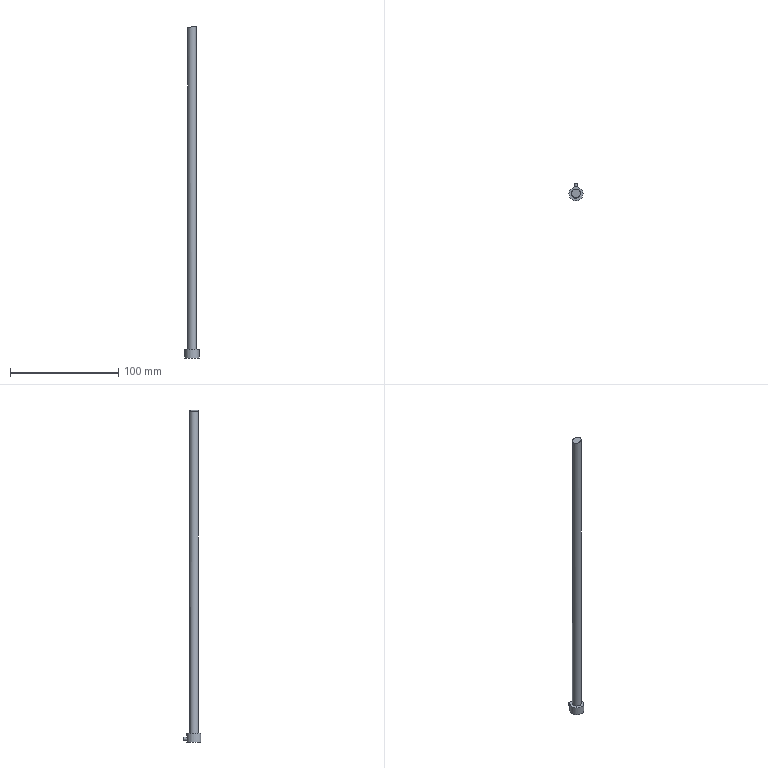Part | STEP file | E108-12-310 | 1 solid | 8 faces | box 13 x 16.5 x 306.86 mm | volume 16065 mm3 | cylinder 3 | plane 3 | spline 1 | cone 1 | commonest cylinder face diameters 3 x1 8 x1 13 x1
STEP:
#1=CARTESIAN_POINT('',(0.,0.,0.));
#2=DIRECTION('',(0.,0.,1.));
#3=DIRECTION('',(1.,0.,0.));
#4=AXIS2_PLACEMENT_3D('',#1,#2,#3);
#5=CARTESIAN_POINT('',(-3.952,0.6196,305.059));
#6=VERTEX_POINT('',#5);
#7=CARTESIAN_POINT('',(-3.952,0.6196,305.059));
#8=CARTESIAN_POINT('',(-4.02,0.1862,305.06));
#9=CARTESIAN_POINT('',(-4.015,-0.2646,305.079));
#10=CARTESIAN_POINT('',(-3.939,-0.6952,305.115));
#11=CARTESIAN_POINT('',(-3.863,-1.126,305.15));
#12=CARTESIAN_POINT('',(-3.714,-1.548,305.203));
#13=CARTESIAN_POINT('',(-3.505,-1.928,305.268));
#14=CARTESIAN_POINT('',(-3.293,-2.313,305.333));
#15=CARTESIAN_POINT('',(-3.015,-2.665,305.413));
#16=CARTESIAN_POINT('',(-2.692,-2.958,305.5));
#17=CARTESIAN_POINT('',(-2.362,-3.259,305.589));
#18=CARTESIAN_POINT('',(-1.976,-3.506,305.688));
#19=CARTESIAN_POINT('',(-1.566,-3.681,305.789));
#20=CARTESIAN_POINT('',(-1.147,-3.859,305.891));
#21=CARTESIAN_POINT('',(-0.6922,-3.966,305.998));
#22=CARTESIAN_POINT('',(-0.2376,-3.993,306.1));
#23=CARTESIAN_POINT('',(0.2209,-4.02,306.203));
#24=CARTESIAN_POINT('',(0.6917,-3.967,306.304));
#25=CARTESIAN_POINT('',(1.135,-3.836,306.395));
#26=CARTESIAN_POINT('',(1.574,-3.706,306.485));
#27=CARTESIAN_POINT('',(1.998,-3.496,306.567));
#28=CARTESIAN_POINT('',(2.37,-3.222,306.635));
#29=CARTESIAN_POINT('',(2.734,-2.954,306.701));
#30=CARTESIAN_POINT('',(3.058,-2.618,306.755));
#31=CARTESIAN_POINT('',(3.313,-2.241,306.793));
#32=CARTESIAN_POINT('',(3.563,-1.872,306.83));
#33=CARTESIAN_POINT('',(3.753,-1.454,306.852));
#34=CARTESIAN_POINT('',(3.867,-1.023,306.858));
#35=CARTESIAN_POINT('',(3.979,-0.5976,306.864));
#36=CARTESIAN_POINT('',(4.021,-0.1473,306.855));
#37=CARTESIAN_POINT('',(3.989,0.2907,306.83));
#38=CARTESIAN_POINT('',(3.958,0.7275,306.806));
#39=CARTESIAN_POINT('',(3.852,1.164,306.767));
#40=CARTESIAN_POINT('',(3.681,1.565,306.716));
#41=CARTESIAN_POINT('',(3.509,1.97,306.664));
#42=CARTESIAN_POINT('',(3.267,2.35,306.599));
#43=CARTESIAN_POINT('',(2.974,2.674,306.525));
#44=CARTESIAN_POINT('',(2.677,3.005,306.449));
#45=CARTESIAN_POINT('',(2.32,3.288,306.363));
#46=CARTESIAN_POINT('',(1.933,3.502,306.272));
#47=CARTESIAN_POINT('',(1.538,3.72,306.179));
#48=CARTESIAN_POINT('',(1.101,3.872,306.078));
#49=CARTESIAN_POINT('',(0.657,3.946,305.978));
#50=CARTESIAN_POINT('',(0.2063,4.021,305.876));
#51=CARTESIAN_POINT('',(-0.2635,4.017,305.772));
#52=CARTESIAN_POINT('',(-0.7138,3.936,305.674));
#53=CARTESIAN_POINT('',(-1.165,3.854,305.576));
#54=CARTESIAN_POINT('',(-1.61,3.691,305.481));
#55=CARTESIAN_POINT('',(-2.01,3.459,305.399));
#56=CARTESIAN_POINT('',(-2.404,3.229,305.317));
#57=CARTESIAN_POINT('',(-2.765,2.926,305.245));
#58=CARTESIAN_POINT('',(-3.062,2.574,305.19));
#59=CARTESIAN_POINT('',(-3.35,2.231,305.136));
#60=CARTESIAN_POINT('',(-3.585,1.831,305.097));
#61=CARTESIAN_POINT('',(-3.744,1.408,305.076));
#62=CARTESIAN_POINT('',(-3.84,1.154,305.064));
#63=CARTESIAN_POINT('',(-3.91,0.8882,305.058));
#64=CARTESIAN_POINT('',(-3.952,0.6196,305.059));
#65=B_SPLINE_CURVE_WITH_KNOTS('',3,(#7,#8,#9,#10,#11,#12,#13,#14,#15,#16,#17,#18,#19,#20,#21,#22,#23,#24,#25,#26,#27,#28,#29,#30,#31,#32,#33,#34,#35,#36,#37,#38,#39,#40,#41,#42,#43,#44,#45,#46,#47,#48,#49,#50,#51,#52,#53,#54,#55,#56,#57,#58,#59,#60,#61,#62,#63,#64),.UNSPECIFIED.,.T.,.F.,(1,3,3,3,3,3,3,3,3,3,3,3,3,3,3,3,3,3,3,3,3,1),(-0.03191,0.,0.05196,0.1039,0.1565,0.2105,0.2658,0.3216,0.3769,0.4311,0.484,0.5361,0.588,0.6405,0.6939,0.7485,0.804,0.8596,0.9145,0.9681,1.,1.052),.UNSPECIFIED.);
#66=CARTESIAN_POINT('',(0.,0.,108.));
#67=DIRECTION('',(0.,0.,-1.));
#68=DIRECTION('',(-1.,0.,0.));
#69=AXIS2_PLACEMENT_3D('',#66,#67,#68);
#70=CYLINDRICAL_SURFACE('',#69,4.);
#71=CARTESIAN_POINT('',(6.439,-197.059));
#72=CARTESIAN_POINT('',(6.415,-197.059));
#73=CARTESIAN_POINT('',(6.367,-197.061));
#74=CARTESIAN_POINT('',(6.294,-197.07));
#75=CARTESIAN_POINT('',(6.222,-197.083));
#76=CARTESIAN_POINT('',(6.15,-197.101));
#77=CARTESIAN_POINT('',(6.078,-197.124));
#78=CARTESIAN_POINT('',(6.006,-197.152));
#79=CARTESIAN_POINT('',(5.934,-197.185));
#80=CARTESIAN_POINT('',(5.862,-197.221));
#81=CARTESIAN_POINT('',(5.79,-197.261));
#82=CARTESIAN_POINT('',(5.719,-197.305));
#83=CARTESIAN_POINT('',(5.648,-197.353));
#84=CARTESIAN_POINT('',(5.576,-197.403));
#85=CARTESIAN_POINT('',(5.505,-197.457));
#86=CARTESIAN_POINT('',(5.435,-197.513));
#87=CARTESIAN_POINT('',(5.364,-197.571));
#88=CARTESIAN_POINT('',(5.293,-197.631));
#89=CARTESIAN_POINT('',(5.222,-197.693));
#90=CARTESIAN_POINT('',(5.152,-197.755));
#91=CARTESIAN_POINT('',(5.081,-197.819));
#92=CARTESIAN_POINT('',(5.011,-197.883));
#93=CARTESIAN_POINT('',(4.94,-197.947));
#94=CARTESIAN_POINT('',(4.87,-198.012));
#95=CARTESIAN_POINT('',(4.799,-198.076));
#96=CARTESIAN_POINT('',(4.729,-198.139));
#97=CARTESIAN_POINT('',(4.658,-198.201));
#98=CARTESIAN_POINT('',(4.588,-198.262));
#99=CARTESIAN_POINT('',(4.517,-198.321));
#100=CARTESIAN_POINT('',(4.446,-198.379));
#101=CARTESIAN_POINT('',(4.375,-198.434));
#102=CARTESIAN_POINT('',(4.304,-198.486));
#103=CARTESIAN_POINT('',(4.233,-198.537));
#104=CARTESIAN_POINT('',(4.162,-198.584));
#105=CARTESIAN_POINT('',(4.09,-198.628));
#106=CARTESIAN_POINT('',(4.019,-198.669));
#107=CARTESIAN_POINT('',(3.947,-198.706));
#108=CARTESIAN_POINT('',(3.875,-198.74));
#109=CARTESIAN_POINT('',(3.803,-198.769));
#110=CARTESIAN_POINT('',(3.732,-198.795));
#111=CARTESIAN_POINT('',(3.66,-198.816));
#112=CARTESIAN_POINT('',(3.587,-198.834));
#113=CARTESIAN_POINT('',(3.515,-198.847));
#114=CARTESIAN_POINT('',(3.443,-198.856));
#115=CARTESIAN_POINT('',(3.371,-198.86));
#116=CARTESIAN_POINT('',(3.298,-198.86));
#117=CARTESIAN_POINT('',(3.226,-198.856));
#118=CARTESIAN_POINT('',(3.153,-198.847));
#119=CARTESIAN_POINT('',(3.081,-198.834));
#120=CARTESIAN_POINT('',(3.009,-198.817));
#121=CARTESIAN_POINT('',(2.937,-198.795));
#122=CARTESIAN_POINT('',(2.865,-198.77));
#123=CARTESIAN_POINT('',(2.793,-198.741));
#124=CARTESIAN_POINT('',(2.721,-198.708));
#125=CARTESIAN_POINT('',(2.65,-198.672));
#126=CARTESIAN_POINT('',(2.578,-198.632));
#127=CARTESIAN_POINT('',(2.506,-198.589));
#128=CARTESIAN_POINT('',(2.435,-198.543));
#129=CARTESIAN_POINT('',(2.364,-198.494));
#130=CARTESIAN_POINT('',(2.293,-198.443));
#131=CARTESIAN_POINT('',(2.221,-198.389));
#132=CARTESIAN_POINT('',(2.15,-198.333));
#133=CARTESIAN_POINT('',(2.08,-198.276));
#134=CARTESIAN_POINT('',(2.009,-198.217));
#135=CARTESIAN_POINT('',(1.938,-198.156));
#136=CARTESIAN_POINT('',(1.868,-198.095));
#137=CARTESIAN_POINT('',(1.797,-198.032));
#138=CARTESIAN_POINT('',(1.727,-197.97));
#139=CARTESIAN_POINT('',(1.656,-197.907));
#140=CARTESIAN_POINT('',(1.585,-197.844));
#141=CARTESIAN_POINT('',(1.515,-197.781));
#142=CARTESIAN_POINT('',(1.444,-197.719));
#143=CARTESIAN_POINT('',(1.374,-197.659));
#144=CARTESIAN_POINT('',(1.303,-197.599));
#145=CARTESIAN_POINT('',(1.232,-197.541));
#146=CARTESIAN_POINT('',(1.161,-197.485));
#147=CARTESIAN_POINT('',(1.09,-197.431));
#148=CARTESIAN_POINT('',(1.019,-197.38));
#149=CARTESIAN_POINT('',(0.9481,-197.332));
#150=CARTESIAN_POINT('',(0.8765,-197.286));
#151=CARTESIAN_POINT('',(0.8049,-197.244));
#152=CARTESIAN_POINT('',(0.7332,-197.206));
#153=CARTESIAN_POINT('',(0.6619,-197.172));
#154=CARTESIAN_POINT('',(0.59,-197.142));
#155=CARTESIAN_POINT('',(0.5178,-197.116));
#156=CARTESIAN_POINT('',(0.4455,-197.094));
#157=CARTESIAN_POINT('',(0.3736,-197.078));
#158=CARTESIAN_POINT('',(0.3011,-197.066));
#159=CARTESIAN_POINT('',(0.2282,-197.059));
#160=CARTESIAN_POINT('',(0.1797,-197.058));
#161=CARTESIAN_POINT('',(0.1555,-197.059));
#162=B_SPLINE_CURVE_WITH_KNOTS('',3,(#71,#72,#73,#74,#75,#76,#77,#78,#79,#80,#81,#82,#83,#84,#85,#86,#87,#88,#89,#90,#91,#92,#93,#94,#95,#96,#97,#98,#99,#100,#101,#102,#103,#104,#105,#106,#107,#108,#109,#110,#111,#112,#113,#114,#115,#116,#117,#118,#119,#120,#121,#122,#123,#124,#125,#126,#127,#128,#129,#130,#131,#132,#133,#134,#135,#136,#137,#138,#139,#140,#141,#142,#143,#144,#145,#146,#147,#148,#149,#150,#151,#152,#153,#154,#155,#156,#157,#158,#159,#160,#161),.UNSPECIFIED.,.F.,.F.,(4,1,1,1,1,1,1,1,1,1,1,1,1,1,1,1,1,1,1,1,1,1,1,1,1,1,1,1,1,1,1,1,1,1,1,1,1,1,1,1,1,1,1,1,1,1,1,1,1,1,1,1,1,1,1,1,1,1,1,1,1,1,1,1,1,1,1,1,1,1,1,1,1,1,1,1,1,1,1,1,1,1,1,1,1,1,1,1,4),(0.,0.01136,0.02273,0.03409,0.04545,0.05682,0.06818,0.07955,0.09091,0.1023,0.1136,0.125,0.1364,0.1477,0.1591,0.1705,0.1818,0.1932,0.2045,0.2159,0.2273,0.2386,0.25,0.2614,0.2727,0.2841,0.2955,0.3068,0.3182,0.3295,0.3409,0.3523,0.3636,0.375,0.3864,0.3977,0.4091,0.4205,0.4318,0.4432,0.4545,0.4659,0.4773,0.4886,0.5,0.5114,0.5227,0.5341,0.5455,0.5568,0.5682,0.5795,0.5909,0.6023,0.6136,0.625,0.6364,0.6477,0.6591,0.6705,0.6818,0.6932,0.7045,0.7159,0.7273,0.7386,0.75,0.7614,0.7727,0.7841,0.7955,0.8068,0.8182,0.8295,0.8409,0.8523,0.8636,0.875,0.8864,0.8977,0.9091,0.9205,0.9318,0.9432,0.9545,0.9659,0.9773,0.9886,1.),.QUASI_UNIFORM_KNOTS.);
#163=(GEOMETRIC_REPRESENTATION_CONTEXT(2)PARAMETRIC_REPRESENTATION_CONTEXT()REPRESENTATION_CONTEXT('',''));
#164=DEFINITIONAL_REPRESENTATION('',(#162),#163);
#165=PCURVE('',#70,#164);
#166=CARTESIAN_POINT('',(-7.07,-15.345,304.943));
#167=CARTESIAN_POINT('',(0.4092,-15.342,306.816));
#168=CARTESIAN_POINT('',(7.936,-15.339,308.349));
#169=CARTESIAN_POINT('',(15.537,-15.336,309.52));
#170=CARTESIAN_POINT('',(-7.049,-4.486,304.509));
#171=CARTESIAN_POINT('',(0.4231,-4.483,306.385));
#172=CARTESIAN_POINT('',(7.941,-4.48,307.92));
#173=CARTESIAN_POINT('',(15.534,-4.477,309.095));
#174=CARTESIAN_POINT('',(-7.039,6.373,304.069));
#175=CARTESIAN_POINT('',(0.4255,6.376,305.948));
#176=CARTESIAN_POINT('',(7.935,6.378,307.486));
#177=CARTESIAN_POINT('',(15.519,6.381,308.665));
#178=CARTESIAN_POINT('',(-7.039,17.231,303.624));
#179=CARTESIAN_POINT('',(0.4166,17.233,305.505));
#180=CARTESIAN_POINT('',(7.918,17.236,307.047));
#181=CARTESIAN_POINT('',(15.493,17.239,308.229));
#182=B_SPLINE_SURFACE_WITH_KNOTS('',3,3,((#166,#167,#168,#169),(#170,#171,#172,#173),(#174,#175,#176,#177),(#178,#179,#180,#181)),.UNSPECIFIED.,.F.,.F.,.F.,(4,4),(4,4),(0.,1.),(0.,1.),.PIECEWISE_BEZIER_KNOTS.);
#183=CARTESIAN_POINT('',(0.49,0.138));
#184=CARTESIAN_POINT('',(0.4871,0.1374));
#185=CARTESIAN_POINT('',(0.4812,0.1364));
#186=CARTESIAN_POINT('',(0.4724,0.1358));
#187=CARTESIAN_POINT('',(0.4635,0.1361));
#188=CARTESIAN_POINT('',(0.4546,0.1373));
#189=CARTESIAN_POINT('',(0.4459,0.1395));
#190=CARTESIAN_POINT('',(0.4374,0.1426));
#191=CARTESIAN_POINT('',(0.4289,0.1466));
#192=CARTESIAN_POINT('',(0.4208,0.1514));
#193=CARTESIAN_POINT('',(0.4129,0.157));
#194=CARTESIAN_POINT('',(0.4053,0.1634));
#195=CARTESIAN_POINT('',(0.3981,0.1706));
#196=CARTESIAN_POINT('',(0.3912,0.1785));
#197=CARTESIAN_POINT('',(0.3847,0.1871));
#198=CARTESIAN_POINT('',(0.3788,0.1963));
#199=CARTESIAN_POINT('',(0.3733,0.206));
#200=CARTESIAN_POINT('',(0.3682,0.2163));
#201=CARTESIAN_POINT('',(0.3637,0.2271));
#202=CARTESIAN_POINT('',(0.3597,0.2383));
#203=CARTESIAN_POINT('',(0.3564,0.2498));
#204=CARTESIAN_POINT('',(0.3535,0.2616));
#205=CARTESIAN_POINT('',(0.3513,0.2738));
#206=CARTESIAN_POINT('',(0.3496,0.2861));
#207=CARTESIAN_POINT('',(0.3485,0.2985));
#208=CARTESIAN_POINT('',(0.3481,0.311));
#209=CARTESIAN_POINT('',(0.3483,0.3236));
#210=CARTESIAN_POINT('',(0.349,0.3361));
#211=CARTESIAN_POINT('',(0.3504,0.3485));
#212=CARTESIAN_POINT('',(0.3524,0.3608));
#213=CARTESIAN_POINT('',(0.355,0.3727));
#214=CARTESIAN_POINT('',(0.3581,0.3845));
#215=CARTESIAN_POINT('',(0.3619,0.3959));
#216=CARTESIAN_POINT('',(0.3662,0.407));
#217=CARTESIAN_POINT('',(0.3711,0.4175));
#218=CARTESIAN_POINT('',(0.3764,0.4275));
#219=CARTESIAN_POINT('',(0.3823,0.437));
#220=CARTESIAN_POINT('',(0.3886,0.4459));
#221=CARTESIAN_POINT('',(0.3954,0.4541));
#222=CARTESIAN_POINT('',(0.4025,0.4616));
#223=CARTESIAN_POINT('',(0.4101,0.4683));
#224=CARTESIAN_POINT('',(0.4179,0.4742));
#225=CARTESIAN_POINT('',(0.4261,0.4793));
#226=CARTESIAN_POINT('',(0.4345,0.4836));
#227=CARTESIAN_POINT('',(0.443,0.4869));
#228=CARTESIAN_POINT('',(0.4517,0.4894));
#229=CARTESIAN_POINT('',(0.4606,0.4909));
#230=CARTESIAN_POINT('',(0.4695,0.4915));
#231=CARTESIAN_POINT('',(0.4783,0.4913));
#232=CARTESIAN_POINT('',(0.4871,0.49));
#233=CARTESIAN_POINT('',(0.4959,0.4879));
#234=CARTESIAN_POINT('',(0.5045,0.4848));
#235=CARTESIAN_POINT('',(0.5129,0.4809));
#236=CARTESIAN_POINT('',(0.5211,0.4761));
#237=CARTESIAN_POINT('',(0.529,0.4705));
#238=CARTESIAN_POINT('',(0.5366,0.4641));
#239=CARTESIAN_POINT('',(0.5439,0.4569));
#240=CARTESIAN_POINT('',(0.5507,0.4491));
#241=CARTESIAN_POINT('',(0.5572,0.4406));
#242=CARTESIAN_POINT('',(0.5632,0.4314));
#243=CARTESIAN_POINT('',(0.5687,0.4216));
#244=CARTESIAN_POINT('',(0.5738,0.4113));
#245=CARTESIAN_POINT('',(0.5783,0.4005));
#246=CARTESIAN_POINT('',(0.5822,0.3894));
#247=CARTESIAN_POINT('',(0.5856,0.3778));
#248=CARTESIAN_POINT('',(0.5885,0.3659));
#249=CARTESIAN_POINT('',(0.5907,0.3537));
#250=CARTESIAN_POINT('',(0.5924,0.3415));
#251=CARTESIAN_POINT('',(0.5934,0.329));
#252=CARTESIAN_POINT('',(0.5938,0.3165));
#253=CARTESIAN_POINT('',(0.5937,0.3039));
#254=CARTESIAN_POINT('',(0.5929,0.2913));
#255=CARTESIAN_POINT('',(0.5915,0.279));
#256=CARTESIAN_POINT('',(0.5895,0.2668));
#257=CARTESIAN_POINT('',(0.5869,0.2547));
#258=CARTESIAN_POINT('',(0.5837,0.2429));
#259=CARTESIAN_POINT('',(0.5799,0.2315));
#260=CARTESIAN_POINT('',(0.5757,0.2205));
#261=CARTESIAN_POINT('',(0.5708,0.21));
#262=CARTESIAN_POINT('',(0.5654,0.1999));
#263=CARTESIAN_POINT('',(0.5596,0.1904));
#264=CARTESIAN_POINT('',(0.5532,0.1815));
#265=CARTESIAN_POINT('',(0.5465,0.1733));
#266=CARTESIAN_POINT('',(0.5394,0.1658));
#267=CARTESIAN_POINT('',(0.5318,0.1591));
#268=CARTESIAN_POINT('',(0.524,0.1531));
#269=CARTESIAN_POINT('',(0.5159,0.148));
#270=CARTESIAN_POINT('',(0.5074,0.1437));
#271=CARTESIAN_POINT('',(0.4988,0.1403));
#272=CARTESIAN_POINT('',(0.493,0.1387));
#273=CARTESIAN_POINT('',(0.49,0.138));
#274=B_SPLINE_CURVE_WITH_KNOTS('',3,(#183,#184,#185,#186,#187,#188,#189,#190,#191,#192,#193,#194,#195,#196,#197,#198,#199,#200,#201,#202,#203,#204,#205,#206,#207,#208,#209,#210,#211,#212,#213,#214,#215,#216,#217,#218,#219,#220,#221,#222,#223,#224,#225,#226,#227,#228,#229,#230,#231,#232,#233,#234,#235,#236,#237,#238,#239,#240,#241,#242,#243,#244,#245,#246,#247,#248,#249,#250,#251,#252,#253,#254,#255,#256,#257,#258,#259,#260,#261,#262,#263,#264,#265,#266,#267,#268,#269,#270,#271,#272,#273),.UNSPECIFIED.,.T.,.F.,(4,1,1,1,1,1,1,1,1,1,1,1,1,1,1,1,1,1,1,1,1,1,1,1,1,1,1,1,1,1,1,1,1,1,1,1,1,1,1,1,1,1,1,1,1,1,1,1,1,1,1,1,1,1,1,1,1,1,1,1,1,1,1,1,1,1,1,1,1,1,1,1,1,1,1,1,1,1,1,1,1,1,1,1,1,1,1,1,4),(0.,0.01136,0.02273,0.03409,0.04545,0.05682,0.06818,0.07955,0.09091,0.1023,0.1136,0.125,0.1364,0.1477,0.1591,0.1705,0.1818,0.1932,0.2045,0.2159,0.2273,0.2386,0.25,0.2614,0.2727,0.2841,0.2955,0.3068,0.3182,0.3295,0.3409,0.3523,0.3636,0.375,0.3864,0.3977,0.4091,0.4205,0.4318,0.4432,0.4545,0.4659,0.4773,0.4886,0.5,0.5114,0.5227,0.5341,0.5455,0.5568,0.5682,0.5795,0.5909,0.6023,0.6136,0.625,0.6364,0.6477,0.6591,0.6705,0.6818,0.6932,0.7045,0.7159,0.7273,0.7386,0.75,0.7614,0.7727,0.7841,0.7955,0.8068,0.8182,0.8295,0.8409,0.8523,0.8636,0.875,0.8864,0.8977,0.9091,0.9205,0.9318,0.9432,0.9545,0.9659,0.9773,0.9886,1.),.QUASI_UNIFORM_KNOTS.);
#275=(GEOMETRIC_REPRESENTATION_CONTEXT(2)PARAMETRIC_REPRESENTATION_CONTEXT()REPRESENTATION_CONTEXT('',''));
#276=DEFINITIONAL_REPRESENTATION('',(#274),#275);
#277=PCURVE('',#182,#276);
#278=SURFACE_CURVE('',#65,(#165,#277),.PCURVE_S1.);
#279=EDGE_CURVE('',#6,#6,#278,.T.);
#280=ORIENTED_EDGE('',*,*,#279,.F.);
#281=CARTESIAN_POINT('',(-3.952,0.6196,8.));
#282=VERTEX_POINT('',#281);
#283=CARTESIAN_POINT('',(-3.952,0.6196,305.059));
#284=CARTESIAN_POINT('',(-3.952,0.6196,8.));
#285=B_SPLINE_CURVE_WITH_KNOTS('',1,(#283,#284),.UNSPECIFIED.,.F.,.F.,(2,2),(-197.059,100.),.PIECEWISE_BEZIER_KNOTS.);
#286=CARTESIAN_POINT('',(6.439,0.));
#287=DIRECTION('',(0.,1.));
#288=VECTOR('',#287,1.);
#289=LINE('',#286,#288);
#290=(GEOMETRIC_REPRESENTATION_CONTEXT(2)PARAMETRIC_REPRESENTATION_CONTEXT()REPRESENTATION_CONTEXT('',''));
#291=DEFINITIONAL_REPRESENTATION('',(#289),#290);
#292=PCURVE('',#70,#291);
#293=CARTESIAN_POINT('',(0.1555,0.));
#294=DIRECTION('',(0.,1.));
#295=VECTOR('',#294,1.);
#296=LINE('',#293,#295);
#297=(GEOMETRIC_REPRESENTATION_CONTEXT(2)PARAMETRIC_REPRESENTATION_CONTEXT()REPRESENTATION_CONTEXT('',''));
#298=DEFINITIONAL_REPRESENTATION('',(#296),#297);
#299=PCURVE('',#70,#298);
#300=SEAM_CURVE('',#285,(#292,#299),.PCURVE_S1.);
#301=EDGE_CURVE('',#6,#282,#300,.T.);
#302=ORIENTED_EDGE('',*,*,#301,.T.);
#303=CARTESIAN_POINT('',(4.,0.,8.));
#304=VERTEX_POINT('',#303);
#305=CARTESIAN_POINT('',(0.,0.,8.));
#306=DIRECTION('',(0.,0.,1.));
#307=DIRECTION('',(1.,0.,0.));
#308=AXIS2_PLACEMENT_3D('',#305,#306,#307);
#309=CIRCLE('',#308,4.);
#310=CARTESIAN_POINT('',(9.425,100.));
#311=DIRECTION('',(-1.,0.));
#312=VECTOR('',#311,1.);
#313=LINE('',#310,#312);
#314=(GEOMETRIC_REPRESENTATION_CONTEXT(2)PARAMETRIC_REPRESENTATION_CONTEXT()REPRESENTATION_CONTEXT('',''));
#315=DEFINITIONAL_REPRESENTATION('',(#313),#314);
#316=PCURVE('',#70,#315);
#317=CARTESIAN_POINT('',(0.,0.,8.));
#318=DIRECTION('',(0.,0.,-1.));
#319=DIRECTION('',(1.,0.,0.));
#320=AXIS2_PLACEMENT_3D('',#317,#318,#319);
#321=PLANE('',#320);
#322=CARTESIAN_POINT('',(4.,0.));
#323=CARTESIAN_POINT('',(4.,-6.928));
#324=CARTESIAN_POINT('',(-2.,-3.464));
#325=CARTESIAN_POINT('',(-8.,0.));
#326=CARTESIAN_POINT('',(-2.,3.464));
#327=CARTESIAN_POINT('',(4.,6.928));
#328=CARTESIAN_POINT('',(4.,0.));
#329=(BOUNDED_CURVE()B_SPLINE_CURVE(2,(#322,#323,#324,#325,#326,#327,#328),.UNSPECIFIED.,.T.,.F.)B_SPLINE_CURVE_WITH_KNOTS((1,2,2,2,2,1),(-2.094,0.,2.094,4.189,6.283,8.378),.UNSPECIFIED.)CURVE()GEOMETRIC_REPRESENTATION_ITEM()RATIONAL_B_SPLINE_CURVE((1.,0.5,1.,0.5,1.,0.5,1.))REPRESENTATION_ITEM(''));
#330=(GEOMETRIC_REPRESENTATION_CONTEXT(2)PARAMETRIC_REPRESENTATION_CONTEXT()REPRESENTATION_CONTEXT('',''));
#331=DEFINITIONAL_REPRESENTATION('',(#329),#330);
#332=PCURVE('',#321,#331);
#333=SURFACE_CURVE('',#309,(#316,#332),.PCURVE_S1.);
#334=EDGE_CURVE('',#282,#304,#333,.T.);
#335=ORIENTED_EDGE('',*,*,#334,.T.);
#336=CARTESIAN_POINT('',(0.,0.,8.));
#337=DIRECTION('',(0.,0.,1.));
#338=DIRECTION('',(1.,0.,0.));
#339=AXIS2_PLACEMENT_3D('',#336,#337,#338);
#340=CIRCLE('',#339,4.);
#341=CARTESIAN_POINT('',(3.142,100.));
#342=DIRECTION('',(-1.,0.));
#343=VECTOR('',#342,1.);
#344=LINE('',#341,#343);
#345=(GEOMETRIC_REPRESENTATION_CONTEXT(2)PARAMETRIC_REPRESENTATION_CONTEXT()REPRESENTATION_CONTEXT('',''));
#346=DEFINITIONAL_REPRESENTATION('',(#344),#345);
#347=PCURVE('',#70,#346);
#348=CARTESIAN_POINT('',(4.,0.));
#349=CARTESIAN_POINT('',(4.,-6.928));
#350=CARTESIAN_POINT('',(-2.,-3.464));
#351=CARTESIAN_POINT('',(-8.,0.));
#352=CARTESIAN_POINT('',(-2.,3.464));
#353=CARTESIAN_POINT('',(4.,6.928));
#354=CARTESIAN_POINT('',(4.,0.));
#355=(BOUNDED_CURVE()B_SPLINE_CURVE(2,(#348,#349,#350,#351,#352,#353,#354),.UNSPECIFIED.,.T.,.F.)B_SPLINE_CURVE_WITH_KNOTS((1,2,2,2,2,1),(-2.094,0.,2.094,4.189,6.283,8.378),.UNSPECIFIED.)CURVE()GEOMETRIC_REPRESENTATION_ITEM()RATIONAL_B_SPLINE_CURVE((1.,0.5,1.,0.5,1.,0.5,1.))REPRESENTATION_ITEM(''));
#356=(GEOMETRIC_REPRESENTATION_CONTEXT(2)PARAMETRIC_REPRESENTATION_CONTEXT()REPRESENTATION_CONTEXT('',''));
#357=DEFINITIONAL_REPRESENTATION('',(#355),#356);
#358=PCURVE('',#321,#357);
#359=SURFACE_CURVE('',#340,(#347,#358),.PCURVE_S1.);
#360=EDGE_CURVE('',#304,#282,#359,.T.);
#361=ORIENTED_EDGE('',*,*,#360,.T.);
#362=ORIENTED_EDGE('',*,*,#301,.F.);
#363=EDGE_LOOP('',(#280,#302,#335,#361,#362));
#364=FACE_BOUND('',#363,.T.);
#365=ADVANCED_FACE('',(#364),#70,.T.);
#366=ORIENTED_EDGE('',*,*,#279,.F.);
#367=EDGE_LOOP('',(#366));
#368=FACE_BOUND('',#367,.F.);
#369=ADVANCED_FACE('',(#368),#182,.F.);
#370=CARTESIAN_POINT('',(6.5,0.,0.));
#371=VERTEX_POINT('',#370);
#372=CARTESIAN_POINT('',(-6.5,0.,0.));
#373=VERTEX_POINT('',#372);
#374=CARTESIAN_POINT('',(0.,0.,0.));
#375=DIRECTION('',(0.,0.,-1.));
#376=DIRECTION('',(-1.,0.,0.));
#377=AXIS2_PLACEMENT_3D('',#374,#375,#376);
#378=CIRCLE('',#377,6.5);
#379=CARTESIAN_POINT('',(0.,0.,8.));
#380=DIRECTION('',(0.,0.,-1.));
#381=DIRECTION('',(1.,0.,0.));
#382=AXIS2_PLACEMENT_3D('',#379,#380,#381);
#383=CYLINDRICAL_SURFACE('',#382,6.5);
#384=CARTESIAN_POINT('',(-3.142,8.));
#385=DIRECTION('',(1.,0.));
#386=VECTOR('',#385,1.);
#387=LINE('',#384,#386);
#388=(GEOMETRIC_REPRESENTATION_CONTEXT(2)PARAMETRIC_REPRESENTATION_CONTEXT()REPRESENTATION_CONTEXT('',''));
#389=DEFINITIONAL_REPRESENTATION('',(#387),#388);
#390=PCURVE('',#383,#389);
#391=CARTESIAN_POINT('',(240.,-1000.,0.));
#392=DIRECTION('',(0.,0.,1.));
#393=DIRECTION('',(-1.,0.,0.));
#394=AXIS2_PLACEMENT_3D('',#391,#392,#393);
#395=PLANE('',#394);
#396=CARTESIAN_POINT('',(246.5,-1000.));
#397=CARTESIAN_POINT('',(246.5,-1011.258));
#398=CARTESIAN_POINT('',(236.75,-1005.629));
#399=CARTESIAN_POINT('',(227.,-1000.));
#400=CARTESIAN_POINT('',(236.75,-994.371));
#401=CARTESIAN_POINT('',(246.5,-988.742));
#402=CARTESIAN_POINT('',(246.5,-1000.));
#403=(BOUNDED_CURVE()B_SPLINE_CURVE(2,(#396,#397,#398,#399,#400,#401,#402),.UNSPECIFIED.,.T.,.F.)B_SPLINE_CURVE_WITH_KNOTS((1,2,2,2,2,1),(-2.094,0.,2.094,4.189,6.283,8.378),.UNSPECIFIED.)CURVE()GEOMETRIC_REPRESENTATION_ITEM()RATIONAL_B_SPLINE_CURVE((1.,0.5,1.,0.5,1.,0.5,1.))REPRESENTATION_ITEM(''));
#404=(GEOMETRIC_REPRESENTATION_CONTEXT(2)PARAMETRIC_REPRESENTATION_CONTEXT()REPRESENTATION_CONTEXT('',''));
#405=DEFINITIONAL_REPRESENTATION('',(#403),#404);
#406=PCURVE('',#395,#405);
#407=SURFACE_CURVE('',#378,(#390,#406),.PCURVE_S1.);
#408=EDGE_CURVE('',#371,#373,#407,.T.);
#409=ORIENTED_EDGE('',*,*,#408,.F.);
#410=CARTESIAN_POINT('',(6.5,0.,8.));
#411=VERTEX_POINT('',#410);
#412=CARTESIAN_POINT('',(6.5,0.,8.));
#413=CARTESIAN_POINT('',(6.5,0.,0.));
#414=B_SPLINE_CURVE_WITH_KNOTS('',1,(#412,#413),.UNSPECIFIED.,.F.,.F.,(2,2),(0.,8.),.PIECEWISE_BEZIER_KNOTS.);
#415=CARTESIAN_POINT('',(0.,0.));
#416=DIRECTION('',(0.,1.));
#417=VECTOR('',#416,1.);
#418=LINE('',#415,#417);
#419=(GEOMETRIC_REPRESENTATION_CONTEXT(2)PARAMETRIC_REPRESENTATION_CONTEXT()REPRESENTATION_CONTEXT('',''));
#420=DEFINITIONAL_REPRESENTATION('',(#418),#419);
#421=PCURVE('',#383,#420);
#422=CARTESIAN_POINT('',(6.283,0.));
#423=DIRECTION('',(0.,1.));
#424=VECTOR('',#423,1.);
#425=LINE('',#422,#424);
#426=(GEOMETRIC_REPRESENTATION_CONTEXT(2)PARAMETRIC_REPRESENTATION_CONTEXT()REPRESENTATION_CONTEXT('',''));
#427=DEFINITIONAL_REPRESENTATION('',(#425),#426);
#428=PCURVE('',#383,#427);
#429=SEAM_CURVE('',#414,(#421,#428),.PCURVE_S1.);
#430=EDGE_CURVE('',#411,#371,#429,.T.);
#431=ORIENTED_EDGE('',*,*,#430,.F.);
#432=CARTESIAN_POINT('',(0.,0.,8.));
#433=DIRECTION('',(0.,0.,-1.));
#434=DIRECTION('',(1.,0.,0.));
#435=AXIS2_PLACEMENT_3D('',#432,#433,#434);
#436=CIRCLE('',#435,6.5);
#437=CARTESIAN_POINT('',(0.,0.));
#438=DIRECTION('',(1.,0.));
#439=VECTOR('',#438,1.);
#440=LINE('',#437,#439);
#441=(GEOMETRIC_REPRESENTATION_CONTEXT(2)PARAMETRIC_REPRESENTATION_CONTEXT()REPRESENTATION_CONTEXT('',''));
#442=DEFINITIONAL_REPRESENTATION('',(#440),#441);
#443=PCURVE('',#383,#442);
#444=CARTESIAN_POINT('',(0.,0.));
#445=DIRECTION('',(1.,0.));
#446=AXIS2_PLACEMENT_2D('',#444,#445);
#447=CIRCLE('',#446,6.5);
#448=(GEOMETRIC_REPRESENTATION_CONTEXT(2)PARAMETRIC_REPRESENTATION_CONTEXT()REPRESENTATION_CONTEXT('',''));
#449=DEFINITIONAL_REPRESENTATION('',(#447),#448);
#450=PCURVE('',#321,#449);
#451=SURFACE_CURVE('',#436,(#443,#450),.PCURVE_S1.);
#452=EDGE_CURVE('',#411,#411,#451,.T.);
#453=ORIENTED_EDGE('',*,*,#452,.T.);
#454=ORIENTED_EDGE('',*,*,#430,.T.);
#455=CARTESIAN_POINT('',(0.,0.,0.));
#456=DIRECTION('',(0.,0.,-1.));
#457=DIRECTION('',(-1.,0.,0.));
#458=AXIS2_PLACEMENT_3D('',#455,#456,#457);
#459=CIRCLE('',#458,6.5);
#460=CARTESIAN_POINT('',(3.142,8.));
#461=DIRECTION('',(1.,0.));
#462=VECTOR('',#461,1.);
#463=LINE('',#460,#462);
#464=(GEOMETRIC_REPRESENTATION_CONTEXT(2)PARAMETRIC_REPRESENTATION_CONTEXT()REPRESENTATION_CONTEXT('',''));
#465=DEFINITIONAL_REPRESENTATION('',(#463),#464);
#466=PCURVE('',#383,#465);
#467=CARTESIAN_POINT('',(246.5,-1000.));
#468=CARTESIAN_POINT('',(246.5,-1011.258));
#469=CARTESIAN_POINT('',(236.75,-1005.629));
#470=CARTESIAN_POINT('',(227.,-1000.));
#471=CARTESIAN_POINT('',(236.75,-994.371));
#472=CARTESIAN_POINT('',(246.5,-988.742));
#473=CARTESIAN_POINT('',(246.5,-1000.));
#474=(BOUNDED_CURVE()B_SPLINE_CURVE(2,(#467,#468,#469,#470,#471,#472,#473),.UNSPECIFIED.,.T.,.F.)B_SPLINE_CURVE_WITH_KNOTS((1,2,2,2,2,1),(-2.094,0.,2.094,4.189,6.283,8.378),.UNSPECIFIED.)CURVE()GEOMETRIC_REPRESENTATION_ITEM()RATIONAL_B_SPLINE_CURVE((1.,0.5,1.,0.5,1.,0.5,1.))REPRESENTATION_ITEM(''));
#475=(GEOMETRIC_REPRESENTATION_CONTEXT(2)PARAMETRIC_REPRESENTATION_CONTEXT()REPRESENTATION_CONTEXT('',''));
#476=DEFINITIONAL_REPRESENTATION('',(#474),#475);
#477=PCURVE('',#395,#476);
#478=SURFACE_CURVE('',#459,(#466,#477),.PCURVE_S1.);
#479=EDGE_CURVE('',#373,#371,#478,.T.);
#480=ORIENTED_EDGE('',*,*,#479,.F.);
#481=EDGE_LOOP('',(#409,#431,#453,#454,#480));
#482=FACE_BOUND('',#481,.T.);
#483=CARTESIAN_POINT('',(0.,6.5,1.5));
#484=VERTEX_POINT('',#483);
#485=CARTESIAN_POINT('',(0.,6.5,1.5));
#486=CARTESIAN_POINT('',(0.1654,6.5,1.5));
#487=CARTESIAN_POINT('',(0.3332,6.493,1.528));
#488=CARTESIAN_POINT('',(0.4892,6.482,1.582));
#489=CARTESIAN_POINT('',(0.6451,6.47,1.636));
#490=CARTESIAN_POINT('',(0.7936,6.453,1.717));
#491=CARTESIAN_POINT('',(0.9231,6.434,1.818));
#492=CARTESIAN_POINT('',(1.055,6.415,1.92));
#493=CARTESIAN_POINT('',(1.17,6.394,2.047));
#494=CARTESIAN_POINT('',(1.261,6.377,2.187));
#495=CARTESIAN_POINT('',(1.352,6.358,2.329));
#496=CARTESIAN_POINT('',(1.421,6.343,2.49));
#497=CARTESIAN_POINT('',(1.46,6.334,2.655));
#498=CARTESIAN_POINT('',(1.498,6.325,2.817));
#499=CARTESIAN_POINT('',(1.509,6.322,2.989));
#500=CARTESIAN_POINT('',(1.492,6.326,3.155));
#501=CARTESIAN_POINT('',(1.475,6.33,3.318));
#502=CARTESIAN_POINT('',(1.431,6.341,3.48));
#503=CARTESIAN_POINT('',(1.362,6.356,3.628));
#504=CARTESIAN_POINT('',(1.293,6.37,3.777));
#505=CARTESIAN_POINT('',(1.199,6.39,3.917));
#506=CARTESIAN_POINT('',(1.085,6.409,4.035));
#507=CARTESIAN_POINT('',(0.9695,6.428,4.157));
#508=CARTESIAN_POINT('',(0.8309,6.448,4.26));
#509=CARTESIAN_POINT('',(0.6809,6.464,4.337));
#510=CARTESIAN_POINT('',(0.5305,6.48,4.413));
#511=CARTESIAN_POINT('',(0.3642,6.492,4.465));
#512=CARTESIAN_POINT('',(0.1962,6.497,4.487));
#513=CARTESIAN_POINT('',(0.03191,6.502,4.509));
#514=CARTESIAN_POINT('',(-0.1386,6.501,4.503));
#515=CARTESIAN_POINT('',(-0.3008,6.493,4.47));
#516=CARTESIAN_POINT('',(-0.4611,6.486,4.437));
#517=CARTESIAN_POINT('',(-0.6177,6.472,4.377));
#518=CARTESIAN_POINT('',(-0.7583,6.456,4.294));
#519=CARTESIAN_POINT('',(-0.9011,6.439,4.211));
#520=CARTESIAN_POINT('',(-1.031,6.419,4.102));
#521=CARTESIAN_POINT('',(-1.139,6.399,3.976));
#522=CARTESIAN_POINT('',(-1.249,6.38,3.848));
#523=CARTESIAN_POINT('',(-1.338,6.361,3.699));
#524=CARTESIAN_POINT('',(-1.399,6.348,3.541));
#525=CARTESIAN_POINT('',(-1.46,6.334,3.384));
#526=CARTESIAN_POINT('',(-1.494,6.326,3.214));
#527=CARTESIAN_POINT('',(-1.499,6.325,3.046));
#528=CARTESIAN_POINT('',(-1.504,6.324,2.881));
#529=CARTESIAN_POINT('',(-1.482,6.329,2.714));
#530=CARTESIAN_POINT('',(-1.433,6.34,2.557));
#531=CARTESIAN_POINT('',(-1.385,6.351,2.4));
#532=CARTESIAN_POINT('',(-1.309,6.367,2.25));
#533=CARTESIAN_POINT('',(-1.214,6.386,2.119));
#534=CARTESIAN_POINT('',(-1.116,6.404,1.984));
#535=CARTESIAN_POINT('',(-0.9937,6.425,1.864));
#536=CARTESIAN_POINT('',(-0.8569,6.443,1.769));
#537=CARTESIAN_POINT('',(-0.7182,6.462,1.672));
#538=CARTESIAN_POINT('',(-0.5604,6.478,1.598));
#539=CARTESIAN_POINT('',(-0.3967,6.488,1.553));
#540=CARTESIAN_POINT('',(-0.2682,6.496,1.518));
#541=CARTESIAN_POINT('',(-0.1335,6.5,1.5));
#542=CARTESIAN_POINT('',(0.,6.5,1.5));
#543=B_SPLINE_CURVE_WITH_KNOTS('',3,(#485,#486,#487,#488,#489,#490,#491,#492,#493,#494,#495,#496,#497,#498,#499,#500,#501,#502,#503,#504,#505,#506,#507,#508,#509,#510,#511,#512,#513,#514,#515,#516,#517,#518,#519,#520,#521,#522,#523,#524,#525,#526,#527,#528,#529,#530,#531,#532,#533,#534,#535,#536,#537,#538,#539,#540,#541,#542),.UNSPECIFIED.,.T.,.F.,(1,3,3,3,3,3,3,3,3,3,3,3,3,3,3,3,3,3,3,3,3,1),(-0.04234,0.,0.05275,0.1054,0.159,0.2132,0.2665,0.3187,0.3713,0.4252,0.4793,0.5321,0.5843,0.6373,0.6915,0.7453,0.7978,0.85,0.9034,0.9577,1.,1.053),.UNSPECIFIED.);
#544=CARTESIAN_POINT('',(4.712,6.5));
#545=CARTESIAN_POINT('',(4.718,6.5));
#546=CARTESIAN_POINT('',(4.729,6.497));
#547=CARTESIAN_POINT('',(4.745,6.486));
#548=CARTESIAN_POINT('',(4.762,6.467));
#549=CARTESIAN_POINT('',(4.778,6.44));
#550=CARTESIAN_POINT('',(4.793,6.406));
#551=CARTESIAN_POINT('',(4.809,6.365));
#552=CARTESIAN_POINT('',(4.823,6.317));
#553=CARTESIAN_POINT('',(4.838,6.262));
#554=CARTESIAN_POINT('',(4.851,6.201));
#555=CARTESIAN_POINT('',(4.864,6.135));
#556=CARTESIAN_POINT('',(4.876,6.062));
#557=CARTESIAN_POINT('',(4.888,5.983));
#558=CARTESIAN_POINT('',(4.898,5.9));
#559=CARTESIAN_POINT('',(4.908,5.813));
#560=CARTESIAN_POINT('',(4.916,5.721));
#561=CARTESIAN_POINT('',(4.924,5.625));
#562=CARTESIAN_POINT('',(4.93,5.526));
#563=CARTESIAN_POINT('',(4.936,5.424));
#564=CARTESIAN_POINT('',(4.94,5.321));
#565=CARTESIAN_POINT('',(4.943,5.215));
#566=CARTESIAN_POINT('',(4.945,5.108));
#567=CARTESIAN_POINT('',(4.945,5.));
#568=CARTESIAN_POINT('',(4.945,4.893));
#569=CARTESIAN_POINT('',(4.943,4.787));
#570=CARTESIAN_POINT('',(4.94,4.681));
#571=CARTESIAN_POINT('',(4.936,4.576));
#572=CARTESIAN_POINT('',(4.93,4.474));
#573=CARTESIAN_POINT('',(4.924,4.376));
#574=CARTESIAN_POINT('',(4.916,4.28));
#575=CARTESIAN_POINT('',(4.908,4.188));
#576=CARTESIAN_POINT('',(4.898,4.1));
#577=CARTESIAN_POINT('',(4.888,4.017));
#578=CARTESIAN_POINT('',(4.877,3.939));
#579=CARTESIAN_POINT('',(4.864,3.866));
#580=CARTESIAN_POINT('',(4.851,3.799));
#581=CARTESIAN_POINT('',(4.838,3.738));
#582=CARTESIAN_POINT('',(4.824,3.683));
#583=CARTESIAN_POINT('',(4.809,3.635));
#584=CARTESIAN_POINT('',(4.793,3.594));
#585=CARTESIAN_POINT('',(4.778,3.56));
#586=CARTESIAN_POINT('',(4.762,3.533));
#587=CARTESIAN_POINT('',(4.745,3.514));
#588=CARTESIAN_POINT('',(4.729,3.503));
#589=CARTESIAN_POINT('',(4.713,3.499));
#590=CARTESIAN_POINT('',(4.696,3.503));
#591=CARTESIAN_POINT('',(4.679,3.514));
#592=CARTESIAN_POINT('',(4.663,3.533));
#593=CARTESIAN_POINT('',(4.647,3.56));
#594=CARTESIAN_POINT('',(4.632,3.594));
#595=CARTESIAN_POINT('',(4.616,3.635));
#596=CARTESIAN_POINT('',(4.601,3.683));
#597=CARTESIAN_POINT('',(4.587,3.737));
#598=CARTESIAN_POINT('',(4.574,3.798));
#599=CARTESIAN_POINT('',(4.561,3.865));
#600=CARTESIAN_POINT('',(4.548,3.938));
#601=CARTESIAN_POINT('',(4.537,4.016));
#602=CARTESIAN_POINT('',(4.527,4.099));
#603=CARTESIAN_POINT('',(4.517,4.187));
#604=CARTESIAN_POINT('',(4.508,4.279));
#605=CARTESIAN_POINT('',(4.501,4.375));
#606=CARTESIAN_POINT('',(4.494,4.473));
#607=CARTESIAN_POINT('',(4.489,4.575));
#608=CARTESIAN_POINT('',(4.485,4.679));
#609=CARTESIAN_POINT('',(4.482,4.785));
#610=CARTESIAN_POINT('',(4.48,4.892));
#611=CARTESIAN_POINT('',(4.479,4.999));
#612=CARTESIAN_POINT('',(4.48,5.106));
#613=CARTESIAN_POINT('',(4.482,5.213));
#614=CARTESIAN_POINT('',(4.485,5.319));
#615=CARTESIAN_POINT('',(4.489,5.423));
#616=CARTESIAN_POINT('',(4.494,5.524));
#617=CARTESIAN_POINT('',(4.501,5.624));
#618=CARTESIAN_POINT('',(4.508,5.72));
#619=CARTESIAN_POINT('',(4.517,5.812));
#620=CARTESIAN_POINT('',(4.526,5.899));
#621=CARTESIAN_POINT('',(4.537,5.982));
#622=CARTESIAN_POINT('',(4.548,6.061));
#623=CARTESIAN_POINT('',(4.56,6.134));
#624=CARTESIAN_POINT('',(4.573,6.201));
#625=CARTESIAN_POINT('',(4.587,6.262));
#626=CARTESIAN_POINT('',(4.601,6.316));
#627=CARTESIAN_POINT('',(4.616,6.364));
#628=CARTESIAN_POINT('',(4.631,6.406));
#629=CARTESIAN_POINT('',(4.647,6.44));
#630=CARTESIAN_POINT('',(4.663,6.466));
#631=CARTESIAN_POINT('',(4.679,6.486));
#632=CARTESIAN_POINT('',(4.696,6.497));
#633=CARTESIAN_POINT('',(4.707,6.5));
#634=CARTESIAN_POINT('',(4.712,6.5));
#635=B_SPLINE_CURVE_WITH_KNOTS('',3,(#544,#545,#546,#547,#548,#549,#550,#551,#552,#553,#554,#555,#556,#557,#558,#559,#560,#561,#562,#563,#564,#565,#566,#567,#568,#569,#570,#571,#572,#573,#574,#575,#576,#577,#578,#579,#580,#581,#582,#583,#584,#585,#586,#587,#588,#589,#590,#591,#592,#593,#594,#595,#596,#597,#598,#599,#600,#601,#602,#603,#604,#605,#606,#607,#608,#609,#610,#611,#612,#613,#614,#615,#616,#617,#618,#619,#620,#621,#622,#623,#624,#625,#626,#627,#628,#629,#630,#631,#632,#633,#634),.UNSPECIFIED.,.T.,.F.,(4,1,1,1,1,1,1,1,1,1,1,1,1,1,1,1,1,1,1,1,1,1,1,1,1,1,1,1,1,1,1,1,1,1,1,1,1,1,1,1,1,1,1,1,1,1,1,1,1,1,1,1,1,1,1,1,1,1,1,1,1,1,1,1,1,1,1,1,1,1,1,1,1,1,1,1,1,1,1,1,1,1,1,1,1,1,1,1,4),(0.,0.01136,0.02273,0.03409,0.04545,0.05682,0.06818,0.07955,0.09091,0.1023,0.1136,0.125,0.1364,0.1477,0.1591,0.1705,0.1818,0.1932,0.2045,0.2159,0.2273,0.2386,0.25,0.2614,0.2727,0.2841,0.2955,0.3068,0.3182,0.3295,0.3409,0.3523,0.3636,0.375,0.3864,0.3977,0.4091,0.4205,0.4318,0.4432,0.4545,0.4659,0.4773,0.4886,0.5,0.5114,0.5227,0.5341,0.5455,0.5568,0.5682,0.5795,0.5909,0.6023,0.6136,0.625,0.6364,0.6477,0.6591,0.6705,0.6818,0.6932,0.7045,0.7159,0.7273,0.7386,0.75,0.7614,0.7727,0.7841,0.7955,0.8068,0.8182,0.8295,0.8409,0.8523,0.8636,0.875,0.8864,0.8977,0.9091,0.9205,0.9318,0.9432,0.9545,0.9659,0.9773,0.9886,1.),.QUASI_UNIFORM_KNOTS.);
#636=(GEOMETRIC_REPRESENTATION_CONTEXT(2)PARAMETRIC_REPRESENTATION_CONTEXT()REPRESENTATION_CONTEXT('',''));
#637=DEFINITIONAL_REPRESENTATION('',(#635),#636);
#638=PCURVE('',#383,#637);
#639=CARTESIAN_POINT('',(0.,2.,3.));
#640=DIRECTION('',(0.,1.,0.));
#641=DIRECTION('',(0.,0.,-1.));
#642=AXIS2_PLACEMENT_3D('',#639,#640,#641);
#643=CYLINDRICAL_SURFACE('',#642,1.5);
#644=CARTESIAN_POINT('',(6.283,4.5));
#645=CARTESIAN_POINT('',(6.259,4.5));
#646=CARTESIAN_POINT('',(6.212,4.499));
#647=CARTESIAN_POINT('',(6.14,4.497));
#648=CARTESIAN_POINT('',(6.068,4.492));
#649=CARTESIAN_POINT('',(5.997,4.486));
#650=CARTESIAN_POINT('',(5.926,4.479));
#651=CARTESIAN_POINT('',(5.854,4.47));
#652=CARTESIAN_POINT('',(5.783,4.46));
#653=CARTESIAN_POINT('',(5.711,4.449));
#654=CARTESIAN_POINT('',(5.64,4.438));
#655=CARTESIAN_POINT('',(5.569,4.425));
#656=CARTESIAN_POINT('',(5.498,4.413));
#657=CARTESIAN_POINT('',(5.427,4.4));
#658=CARTESIAN_POINT('',(5.355,4.388));
#659=CARTESIAN_POINT('',(5.284,4.376));
#660=CARTESIAN_POINT('',(5.213,4.365));
#661=CARTESIAN_POINT('',(5.142,4.355));
#662=CARTESIAN_POINT('',(5.07,4.346));
#663=CARTESIAN_POINT('',(4.999,4.338));
#664=CARTESIAN_POINT('',(4.928,4.332));
#665=CARTESIAN_POINT('',(4.856,4.328));
#666=CARTESIAN_POINT('',(4.784,4.325));
#667=CARTESIAN_POINT('',(4.713,4.324));
#668=CARTESIAN_POINT('',(4.641,4.325));
#669=CARTESIAN_POINT('',(4.57,4.328));
#670=CARTESIAN_POINT('',(4.498,4.332));
#671=CARTESIAN_POINT('',(4.426,4.339));
#672=CARTESIAN_POINT('',(4.355,4.346));
#673=CARTESIAN_POINT('',(4.283,4.355));
#674=CARTESIAN_POINT('',(4.212,4.365));
#675=CARTESIAN_POINT('',(4.141,4.376));
#676=CARTESIAN_POINT('',(4.07,4.388));
#677=CARTESIAN_POINT('',(3.998,4.4));
#678=CARTESIAN_POINT('',(3.927,4.413));
#679=CARTESIAN_POINT('',(3.856,4.425));
#680=CARTESIAN_POINT('',(3.785,4.437));
#681=CARTESIAN_POINT('',(3.714,4.449));
#682=CARTESIAN_POINT('',(3.642,4.46));
#683=CARTESIAN_POINT('',(3.571,4.47));
#684=CARTESIAN_POINT('',(3.5,4.479));
#685=CARTESIAN_POINT('',(3.428,4.486));
#686=CARTESIAN_POINT('',(3.357,4.492));
#687=CARTESIAN_POINT('',(3.285,4.497));
#688=CARTESIAN_POINT('',(3.214,4.499));
#689=CARTESIAN_POINT('',(3.142,4.5));
#690=CARTESIAN_POINT('',(3.07,4.499));
#691=CARTESIAN_POINT('',(2.999,4.497));
#692=CARTESIAN_POINT('',(2.927,4.492));
#693=CARTESIAN_POINT('',(2.856,4.486));
#694=CARTESIAN_POINT('',(2.784,4.479));
#695=CARTESIAN_POINT('',(2.713,4.47));
#696=CARTESIAN_POINT('',(2.641,4.46));
#697=CARTESIAN_POINT('',(2.57,4.449));
#698=CARTESIAN_POINT('',(2.499,4.438));
#699=CARTESIAN_POINT('',(2.428,4.425));
#700=CARTESIAN_POINT('',(2.357,4.413));
#701=CARTESIAN_POINT('',(2.285,4.4));
#702=CARTESIAN_POINT('',(2.215,4.388));
#703=CARTESIAN_POINT('',(2.143,4.376));
#704=CARTESIAN_POINT('',(2.072,4.365));
#705=CARTESIAN_POINT('',(2.,4.355));
#706=CARTESIAN_POINT('',(1.929,4.346));
#707=CARTESIAN_POINT('',(1.858,4.339));
#708=CARTESIAN_POINT('',(1.786,4.332));
#709=CARTESIAN_POINT('',(1.715,4.328));
#710=CARTESIAN_POINT('',(1.643,4.325));
#711=CARTESIAN_POINT('',(1.572,4.324));
#712=CARTESIAN_POINT('',(1.5,4.325));
#713=CARTESIAN_POINT('',(1.428,4.328));
#714=CARTESIAN_POINT('',(1.357,4.332));
#715=CARTESIAN_POINT('',(1.285,4.338));
#716=CARTESIAN_POINT('',(1.214,4.346));
#717=CARTESIAN_POINT('',(1.142,4.355));
#718=CARTESIAN_POINT('',(1.071,4.365));
#719=CARTESIAN_POINT('',(0.9995,4.376));
#720=CARTESIAN_POINT('',(0.9286,4.388));
#721=CARTESIAN_POINT('',(0.8575,4.4));
#722=CARTESIAN_POINT('',(0.7862,4.413));
#723=CARTESIAN_POINT('',(0.7149,4.425));
#724=CARTESIAN_POINT('',(0.6436,4.437));
#725=CARTESIAN_POINT('',(0.5728,4.449));
#726=CARTESIAN_POINT('',(0.5015,4.46));
#727=CARTESIAN_POINT('',(0.43,4.47));
#728=CARTESIAN_POINT('',(0.3585,4.479));
#729=CARTESIAN_POINT('',(0.2872,4.486));
#730=CARTESIAN_POINT('',(0.2157,4.492));
#731=CARTESIAN_POINT('',(0.1438,4.497));
#732=CARTESIAN_POINT('',(0.07178,4.499));
#733=CARTESIAN_POINT('',(0.02388,4.5));
#734=CARTESIAN_POINT('',(0.,4.5));
#735=B_SPLINE_CURVE_WITH_KNOTS('',3,(#644,#645,#646,#647,#648,#649,#650,#651,#652,#653,#654,#655,#656,#657,#658,#659,#660,#661,#662,#663,#664,#665,#666,#667,#668,#669,#670,#671,#672,#673,#674,#675,#676,#677,#678,#679,#680,#681,#682,#683,#684,#685,#686,#687,#688,#689,#690,#691,#692,#693,#694,#695,#696,#697,#698,#699,#700,#701,#702,#703,#704,#705,#706,#707,#708,#709,#710,#711,#712,#713,#714,#715,#716,#717,#718,#719,#720,#721,#722,#723,#724,#725,#726,#727,#728,#729,#730,#731,#732,#733,#734),.UNSPECIFIED.,.F.,.F.,(4,1,1,1,1,1,1,1,1,1,1,1,1,1,1,1,1,1,1,1,1,1,1,1,1,1,1,1,1,1,1,1,1,1,1,1,1,1,1,1,1,1,1,1,1,1,1,1,1,1,1,1,1,1,1,1,1,1,1,1,1,1,1,1,1,1,1,1,1,1,1,1,1,1,1,1,1,1,1,1,1,1,1,1,1,1,1,1,4),(0.,0.01136,0.02273,0.03409,0.04545,0.05682,0.06818,0.07955,0.09091,0.1023,0.1136,0.125,0.1364,0.1477,0.1591,0.1705,0.1818,0.1932,0.2045,0.2159,0.2273,0.2386,0.25,0.2614,0.2727,0.2841,0.2955,0.3068,0.3182,0.3295,0.3409,0.3523,0.3636,0.375,0.3864,0.3977,0.4091,0.4205,0.4318,0.4432,0.4545,0.4659,0.4773,0.4886,0.5,0.5114,0.5227,0.5341,0.5455,0.5568,0.5682,0.5795,0.5909,0.6023,0.6136,0.625,0.6364,0.6477,0.6591,0.6705,0.6818,0.6932,0.7045,0.7159,0.7273,0.7386,0.75,0.7614,0.7727,0.7841,0.7955,0.8068,0.8182,0.8295,0.8409,0.8523,0.8636,0.875,0.8864,0.8977,0.9091,0.9205,0.9318,0.9432,0.9545,0.9659,0.9773,0.9886,1.),.QUASI_UNIFORM_KNOTS.);
#736=(GEOMETRIC_REPRESENTATION_CONTEXT(2)PARAMETRIC_REPRESENTATION_CONTEXT()REPRESENTATION_CONTEXT('',''));
#737=DEFINITIONAL_REPRESENTATION('',(#735),#736);
#738=PCURVE('',#643,#737);
#739=SURFACE_CURVE('',#543,(#638,#738),.PCURVE_S1.);
#740=EDGE_CURVE('',#484,#484,#739,.T.);
#741=ORIENTED_EDGE('',*,*,#740,.T.);
#742=EDGE_LOOP('',(#741));
#743=FACE_BOUND('',#742,.T.);
#744=ADVANCED_FACE('',(#482,#743),#383,.T.);
#745=ORIENTED_EDGE('',*,*,#360,.F.);
#746=ORIENTED_EDGE('',*,*,#334,.F.);
#747=EDGE_LOOP('',(#745,#746));
#748=FACE_BOUND('',#747,.T.);
#749=ORIENTED_EDGE('',*,*,#452,.F.);
#750=EDGE_LOOP('',(#749));
#751=FACE_BOUND('',#750,.T.);
#752=ADVANCED_FACE('',(#748,#751),#321,.F.);
#753=ORIENTED_EDGE('',*,*,#479,.T.);
#754=ORIENTED_EDGE('',*,*,#408,.T.);
#755=EDGE_LOOP('',(#753,#754));
#756=FACE_BOUND('',#755,.T.);
#757=ADVANCED_FACE('',(#756),#395,.F.);
#758=CARTESIAN_POINT('',(0.,10.,1.75));
#759=VERTEX_POINT('',#758);
#760=CARTESIAN_POINT('',(0.,10.,3.));
#761=DIRECTION('',(0.,1.,0.));
#762=DIRECTION('',(0.,0.,-1.));
#763=AXIS2_PLACEMENT_3D('',#760,#761,#762);
#764=CIRCLE('',#763,1.25);
#765=CARTESIAN_POINT('',(0.,10.,3.));
#766=DIRECTION('',(0.,1.,0.));
#767=DIRECTION('',(0.,0.,-1.));
#768=AXIS2_PLACEMENT_3D('',#765,#766,#767);
#769=PLANE('',#768);
#770=CARTESIAN_POINT('',(0.,0.));
#771=DIRECTION('',(1.,0.));
#772=AXIS2_PLACEMENT_2D('',#770,#771);
#773=CIRCLE('',#772,1.25);
#774=(GEOMETRIC_REPRESENTATION_CONTEXT(2)PARAMETRIC_REPRESENTATION_CONTEXT()REPRESENTATION_CONTEXT('',''));
#775=DEFINITIONAL_REPRESENTATION('',(#773),#774);
#776=PCURVE('',#769,#775);
#777=CARTESIAN_POINT('',(0.,9.75,3.));
#778=DIRECTION('',(0.,-1.,0.));
#779=DIRECTION('',(0.,0.,1.));
#780=AXIS2_PLACEMENT_3D('',#777,#778,#779);
#781=CONICAL_SURFACE('',#780,1.5,0.7854);
#782=CARTESIAN_POINT('',(9.425,-0.25));
#783=DIRECTION('',(-1.,0.));
#784=VECTOR('',#783,1.);
#785=LINE('',#782,#784);
#786=(GEOMETRIC_REPRESENTATION_CONTEXT(2)PARAMETRIC_REPRESENTATION_CONTEXT()REPRESENTATION_CONTEXT('',''));
#787=DEFINITIONAL_REPRESENTATION('',(#785),#786);
#788=PCURVE('',#781,#787);
#789=SURFACE_CURVE('',#764,(#776,#788),.PCURVE_S1.);
#790=EDGE_CURVE('',#759,#759,#789,.T.);
#791=ORIENTED_EDGE('',*,*,#790,.T.);
#792=EDGE_LOOP('',(#791));
#793=FACE_BOUND('',#792,.T.);
#794=ADVANCED_FACE('',(#793),#769,.T.);
#795=ORIENTED_EDGE('',*,*,#790,.F.);
#796=CARTESIAN_POINT('',(0.,9.75,1.5));
#797=VERTEX_POINT('',#796);
#798=CARTESIAN_POINT('',(0.,10.,1.75));
#799=CARTESIAN_POINT('',(0.,9.75,1.5));
#800=B_SPLINE_CURVE_WITH_KNOTS('',1,(#798,#799),.UNSPECIFIED.,.F.,.F.,(2,2),(-0.3536,0.),.PIECEWISE_BEZIER_KNOTS.);
#801=CARTESIAN_POINT('',(9.425,0.));
#802=DIRECTION('',(0.,1.));
#803=VECTOR('',#802,1.);
#804=LINE('',#801,#803);
#805=(GEOMETRIC_REPRESENTATION_CONTEXT(2)PARAMETRIC_REPRESENTATION_CONTEXT()REPRESENTATION_CONTEXT('',''));
#806=DEFINITIONAL_REPRESENTATION('',(#804),#805);
#807=PCURVE('',#781,#806);
#808=CARTESIAN_POINT('',(3.142,0.));
#809=DIRECTION('',(0.,1.));
#810=VECTOR('',#809,1.);
#811=LINE('',#808,#810);
#812=(GEOMETRIC_REPRESENTATION_CONTEXT(2)PARAMETRIC_REPRESENTATION_CONTEXT()REPRESENTATION_CONTEXT('',''));
#813=DEFINITIONAL_REPRESENTATION('',(#811),#812);
#814=PCURVE('',#781,#813);
#815=SEAM_CURVE('',#800,(#807,#814),.PCURVE_S1.);
#816=EDGE_CURVE('',#759,#797,#815,.T.);
#817=ORIENTED_EDGE('',*,*,#816,.T.);
#818=CARTESIAN_POINT('',(0.,9.75,3.));
#819=DIRECTION('',(0.,-1.,0.));
#820=DIRECTION('',(0.,0.,-1.));
#821=AXIS2_PLACEMENT_3D('',#818,#819,#820);
#822=CIRCLE('',#821,1.5);
#823=CARTESIAN_POINT('',(3.142,0.));
#824=DIRECTION('',(1.,0.));
#825=VECTOR('',#824,1.);
#826=LINE('',#823,#825);
#827=(GEOMETRIC_REPRESENTATION_CONTEXT(2)PARAMETRIC_REPRESENTATION_CONTEXT()REPRESENTATION_CONTEXT('',''));
#828=DEFINITIONAL_REPRESENTATION('',(#826),#827);
#829=PCURVE('',#781,#828);
#830=CARTESIAN_POINT('',(6.283,7.75));
#831=DIRECTION('',(-1.,0.));
#832=VECTOR('',#831,1.);
#833=LINE('',#830,#832);
#834=(GEOMETRIC_REPRESENTATION_CONTEXT(2)PARAMETRIC_REPRESENTATION_CONTEXT()REPRESENTATION_CONTEXT('',''));
#835=DEFINITIONAL_REPRESENTATION('',(#833),#834);
#836=PCURVE('',#643,#835);
#837=SURFACE_CURVE('',#822,(#829,#836),.PCURVE_S1.);
#838=EDGE_CURVE('',#797,#797,#837,.T.);
#839=ORIENTED_EDGE('',*,*,#838,.F.);
#840=ORIENTED_EDGE('',*,*,#816,.F.);
#841=EDGE_LOOP('',(#795,#817,#839,#840));
#842=FACE_BOUND('',#841,.T.);
#843=ADVANCED_FACE('',(#842),#781,.T.);
#844=ORIENTED_EDGE('',*,*,#740,.F.);
#845=CARTESIAN_POINT('',(0.,6.5,1.5));
#846=CARTESIAN_POINT('',(0.,9.75,1.5));
#847=B_SPLINE_CURVE_WITH_KNOTS('',1,(#845,#846),.UNSPECIFIED.,.F.,.F.,(2,2),(4.5,7.75),.PIECEWISE_BEZIER_KNOTS.);
#848=CARTESIAN_POINT('',(6.283,0.));
#849=DIRECTION('',(0.,1.));
#850=VECTOR('',#849,1.);
#851=LINE('',#848,#850);
#852=(GEOMETRIC_REPRESENTATION_CONTEXT(2)PARAMETRIC_REPRESENTATION_CONTEXT()REPRESENTATION_CONTEXT('',''));
#853=DEFINITIONAL_REPRESENTATION('',(#851),#852);
#854=PCURVE('',#643,#853);
#855=CARTESIAN_POINT('',(0.,0.));
#856=DIRECTION('',(0.,1.));
#857=VECTOR('',#856,1.);
#858=LINE('',#855,#857);
#859=(GEOMETRIC_REPRESENTATION_CONTEXT(2)PARAMETRIC_REPRESENTATION_CONTEXT()REPRESENTATION_CONTEXT('',''));
#860=DEFINITIONAL_REPRESENTATION('',(#858),#859);
#861=PCURVE('',#643,#860);
#862=SEAM_CURVE('',#847,(#854,#861),.PCURVE_S1.);
#863=EDGE_CURVE('',#484,#797,#862,.T.);
#864=ORIENTED_EDGE('',*,*,#863,.T.);
#865=ORIENTED_EDGE('',*,*,#838,.T.);
#866=ORIENTED_EDGE('',*,*,#863,.F.);
#867=EDGE_LOOP('',(#844,#864,#865,#866));
#868=FACE_BOUND('',#867,.T.);
#869=ADVANCED_FACE('',(#868),#643,.T.);
#870=CLOSED_SHELL('',(#365,#369,#744,#752,#757,#794,#843,#869));
#871=MANIFOLD_SOLID_BREP('',#870);
#872=(LENGTH_UNIT()NAMED_UNIT(*)SI_UNIT(.MILLI.,.METRE.));
#873=UNCERTAINTY_MEASURE_WITH_UNIT(LENGTH_MEASURE(0.00005),#872,'','');
#874=(NAMED_UNIT(*)PLANE_ANGLE_UNIT()SI_UNIT($,.RADIAN.));
#875=(NAMED_UNIT(*)SI_UNIT($,.STERADIAN.)SOLID_ANGLE_UNIT());
#876=(GEOMETRIC_REPRESENTATION_CONTEXT(3)GLOBAL_UNCERTAINTY_ASSIGNED_CONTEXT((#873))GLOBAL_UNIT_ASSIGNED_CONTEXT((#872,#874,#875))REPRESENTATION_CONTEXT('',''));
#877=ADVANCED_BREP_SHAPE_REPRESENTATION('',(#4,#871),#876);